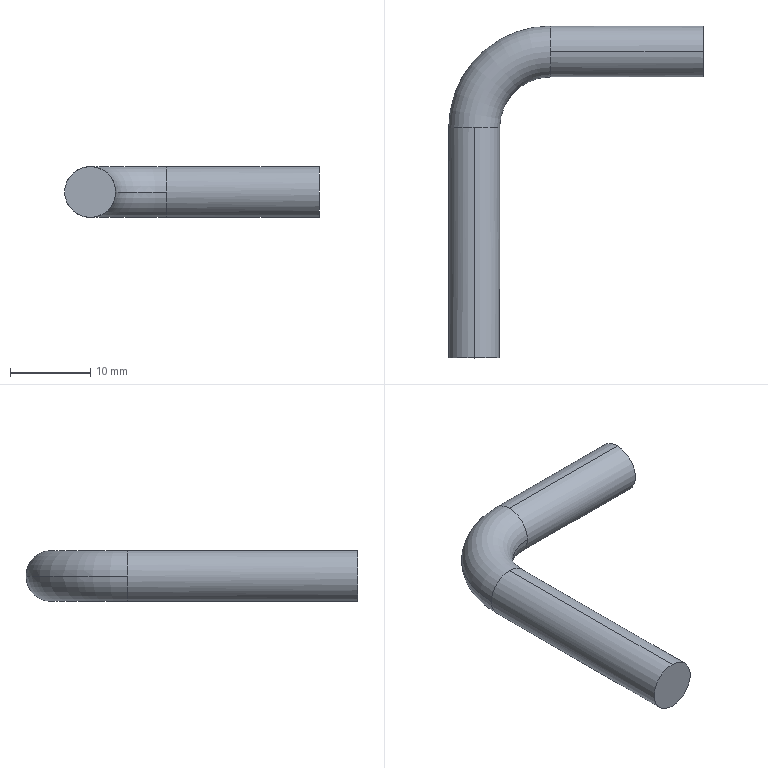Part | SolidWorks | features Sweep 1 | 1 solid | 8 faces | box 31.75 x 41.402 x 6.35 mm | volume 1986 mm3 | cylinder 4 | torus 2 | plane 2 | commonest cylinder face diameters 6.35 x4
STEP:
#1=CARTESIAN_POINT('',(0.,1.13,-0.125));
#2=VERTEX_POINT('',#1);
#3=CARTESIAN_POINT('',(-0.125,1.13,0.));
#4=VERTEX_POINT('',#3);
#5=CARTESIAN_POINT('',(0.,1.13,0.));
#6=DIRECTION('',(0.,1.,0.));
#7=DIRECTION('',(0.,0.,1.));
#8=AXIS2_PLACEMENT_3D('',#5,#6,#7);
#9=CIRCLE('',#8,0.125);
#10=EDGE_CURVE('',#2,#4,#9,.T.);
#11=ORIENTED_EDGE('',*,*,#10,.T.);
#12=CARTESIAN_POINT('',(0.375,1.63,0.));
#13=VERTEX_POINT('',#12);
#14=CARTESIAN_POINT('',(0.375,1.13,0.));
#15=DIRECTION('',(0.,0.,-1.));
#16=DIRECTION('',(-1.,0.,0.));
#17=AXIS2_PLACEMENT_3D('',#14,#15,#16);
#18=CIRCLE('',#17,0.5);
#19=EDGE_CURVE('',#4,#13,#18,.T.);
#20=ORIENTED_EDGE('',*,*,#19,.T.);
#21=CARTESIAN_POINT('',(0.375,1.505,-0.125));
#22=VERTEX_POINT('',#21);
#23=CARTESIAN_POINT('',(0.375,1.505,0.));
#24=DIRECTION('',(1.,0.,0.));
#25=DIRECTION('',(0.,0.,1.));
#26=AXIS2_PLACEMENT_3D('',#23,#24,#25);
#27=CIRCLE('',#26,0.125);
#28=EDGE_CURVE('',#22,#13,#27,.T.);
#29=ORIENTED_EDGE('',*,*,#28,.F.);
#30=CARTESIAN_POINT('',(0.375,1.38,0.));
#31=VERTEX_POINT('',#30);
#32=CARTESIAN_POINT('',(0.375,1.505,0.));
#33=DIRECTION('',(1.,0.,0.));
#34=DIRECTION('',(0.,0.,1.));
#35=AXIS2_PLACEMENT_3D('',#32,#33,#34);
#36=CIRCLE('',#35,0.125);
#37=EDGE_CURVE('',#31,#22,#36,.T.);
#38=ORIENTED_EDGE('',*,*,#37,.F.);
#39=CARTESIAN_POINT('',(0.125,1.13,0.));
#40=VERTEX_POINT('',#39);
#41=CARTESIAN_POINT('',(0.375,1.13,0.));
#42=DIRECTION('',(0.,0.,-1.));
#43=DIRECTION('',(-1.,0.,0.));
#44=AXIS2_PLACEMENT_3D('',#41,#42,#43);
#45=CIRCLE('',#44,0.25);
#46=EDGE_CURVE('',#40,#31,#45,.T.);
#47=ORIENTED_EDGE('',*,*,#46,.F.);
#48=CARTESIAN_POINT('',(0.,1.13,0.));
#49=DIRECTION('',(0.,1.,0.));
#50=DIRECTION('',(0.,0.,1.));
#51=AXIS2_PLACEMENT_3D('',#48,#49,#50);
#52=CIRCLE('',#51,0.125);
#53=EDGE_CURVE('',#40,#2,#52,.T.);
#54=ORIENTED_EDGE('',*,*,#53,.T.);
#55=EDGE_LOOP('',(#11,#20,#29,#38,#47,#54));
#56=FACE_OUTER_BOUND('',#55,.T.);
#57=CARTESIAN_POINT('',(0.375,1.13,0.));
#58=DIRECTION('',(0.,0.,-1.));
#59=DIRECTION('',(-1.,0.,0.));
#60=AXIS2_PLACEMENT_3D('',#57,#58,#59);
#61=TOROIDAL_SURFACE('',#60,0.375,0.125);
#62=ADVANCED_FACE('',(#56),#61,.T.);
#63=CARTESIAN_POINT('',(0.,1.13,0.125));
#64=VERTEX_POINT('',#63);
#65=CARTESIAN_POINT('',(0.,1.13,0.));
#66=DIRECTION('',(0.,1.,0.));
#67=DIRECTION('',(0.,0.,1.));
#68=AXIS2_PLACEMENT_3D('',#65,#66,#67);
#69=CIRCLE('',#68,0.125);
#70=EDGE_CURVE('',#64,#40,#69,.T.);
#71=ORIENTED_EDGE('',*,*,#70,.F.);
#72=CARTESIAN_POINT('',(0.,0.,0.125));
#73=VERTEX_POINT('',#72);
#74=CARTESIAN_POINT('',(0.,1.13,0.125));
#75=DIRECTION('',(0.,-1.,0.));
#76=VECTOR('',#75,39.37);
#77=LINE('',#74,#76);
#78=EDGE_CURVE('',#64,#73,#77,.T.);
#79=ORIENTED_EDGE('',*,*,#78,.T.);
#80=CARTESIAN_POINT('',(0.,0.,-0.125));
#81=VERTEX_POINT('',#80);
#82=CARTESIAN_POINT('',(0.,0.,0.));
#83=DIRECTION('',(0.,1.,0.));
#84=DIRECTION('',(0.,0.,1.));
#85=AXIS2_PLACEMENT_3D('',#82,#83,#84);
#86=CIRCLE('',#85,0.125);
#87=EDGE_CURVE('',#73,#81,#86,.T.);
#88=ORIENTED_EDGE('',*,*,#87,.T.);
#89=CARTESIAN_POINT('',(0.,1.13,-0.125));
#90=DIRECTION('',(0.,-1.,0.));
#91=VECTOR('',#90,39.37);
#92=LINE('',#89,#91);
#93=EDGE_CURVE('',#2,#81,#92,.T.);
#94=ORIENTED_EDGE('',*,*,#93,.F.);
#95=ORIENTED_EDGE('',*,*,#53,.F.);
#96=EDGE_LOOP('',(#71,#79,#88,#94,#95));
#97=FACE_OUTER_BOUND('',#96,.T.);
#98=CARTESIAN_POINT('',(0.,1.13,0.));
#99=DIRECTION('',(0.,-1.,0.));
#100=DIRECTION('',(0.,0.,-1.));
#101=AXIS2_PLACEMENT_3D('',#98,#99,#100);
#102=CYLINDRICAL_SURFACE('',#101,0.125);
#103=ADVANCED_FACE('',(#97),#102,.T.);
#104=ORIENTED_EDGE('',*,*,#28,.T.);
#105=CARTESIAN_POINT('',(0.375,1.505,0.125));
#106=VERTEX_POINT('',#105);
#107=CARTESIAN_POINT('',(0.375,1.505,0.));
#108=DIRECTION('',(1.,0.,0.));
#109=DIRECTION('',(0.,0.,1.));
#110=AXIS2_PLACEMENT_3D('',#107,#108,#109);
#111=CIRCLE('',#110,0.125);
#112=EDGE_CURVE('',#13,#106,#111,.T.);
#113=ORIENTED_EDGE('',*,*,#112,.T.);
#114=CARTESIAN_POINT('',(1.125,1.505,0.125));
#115=VERTEX_POINT('',#114);
#116=CARTESIAN_POINT('',(0.375,1.505,0.125));
#117=DIRECTION('',(1.,0.,0.));
#118=VECTOR('',#117,39.37);
#119=LINE('',#116,#118);
#120=EDGE_CURVE('',#106,#115,#119,.T.);
#121=ORIENTED_EDGE('',*,*,#120,.T.);
#122=CARTESIAN_POINT('',(1.125,1.505,-0.125));
#123=VERTEX_POINT('',#122);
#124=CARTESIAN_POINT('',(1.125,1.505,0.));
#125=DIRECTION('',(1.,0.,0.));
#126=DIRECTION('',(0.,0.,1.));
#127=AXIS2_PLACEMENT_3D('',#124,#125,#126);
#128=CIRCLE('',#127,0.125);
#129=EDGE_CURVE('',#123,#115,#128,.T.);
#130=ORIENTED_EDGE('',*,*,#129,.F.);
#131=CARTESIAN_POINT('',(0.375,1.505,-0.125));
#132=DIRECTION('',(1.,0.,0.));
#133=VECTOR('',#132,39.37);
#134=LINE('',#131,#133);
#135=EDGE_CURVE('',#22,#123,#134,.T.);
#136=ORIENTED_EDGE('',*,*,#135,.F.);
#137=EDGE_LOOP('',(#104,#113,#121,#130,#136));
#138=FACE_OUTER_BOUND('',#137,.T.);
#139=CARTESIAN_POINT('',(0.375,1.505,0.));
#140=DIRECTION('',(1.,0.,0.));
#141=DIRECTION('',(0.,0.,-1.));
#142=AXIS2_PLACEMENT_3D('',#139,#140,#141);
#143=CYLINDRICAL_SURFACE('',#142,0.125);
#144=ADVANCED_FACE('',(#138),#143,.T.);
#145=ORIENTED_EDGE('',*,*,#120,.F.);
#146=CARTESIAN_POINT('',(0.375,1.505,0.));
#147=DIRECTION('',(1.,0.,0.));
#148=DIRECTION('',(0.,0.,1.));
#149=AXIS2_PLACEMENT_3D('',#146,#147,#148);
#150=CIRCLE('',#149,0.125);
#151=EDGE_CURVE('',#106,#31,#150,.T.);
#152=ORIENTED_EDGE('',*,*,#151,.T.);
#153=ORIENTED_EDGE('',*,*,#37,.T.);
#154=ORIENTED_EDGE('',*,*,#135,.T.);
#155=CARTESIAN_POINT('',(1.125,1.505,0.));
#156=DIRECTION('',(1.,0.,0.));
#157=DIRECTION('',(0.,0.,1.));
#158=AXIS2_PLACEMENT_3D('',#155,#156,#157);
#159=CIRCLE('',#158,0.125);
#160=EDGE_CURVE('',#115,#123,#159,.T.);
#161=ORIENTED_EDGE('',*,*,#160,.F.);
#162=EDGE_LOOP('',(#145,#152,#153,#154,#161));
#163=FACE_OUTER_BOUND('',#162,.T.);
#164=CARTESIAN_POINT('',(0.375,1.505,0.));
#165=DIRECTION('',(1.,0.,0.));
#166=DIRECTION('',(0.,0.,-1.));
#167=AXIS2_PLACEMENT_3D('',#164,#165,#166);
#168=CYLINDRICAL_SURFACE('',#167,0.125);
#169=ADVANCED_FACE('',(#163),#168,.T.);
#170=ORIENTED_EDGE('',*,*,#19,.F.);
#171=CARTESIAN_POINT('',(0.,1.13,0.));
#172=DIRECTION('',(0.,1.,0.));
#173=DIRECTION('',(0.,0.,1.));
#174=AXIS2_PLACEMENT_3D('',#171,#172,#173);
#175=CIRCLE('',#174,0.125);
#176=EDGE_CURVE('',#4,#64,#175,.T.);
#177=ORIENTED_EDGE('',*,*,#176,.T.);
#178=ORIENTED_EDGE('',*,*,#70,.T.);
#179=ORIENTED_EDGE('',*,*,#46,.T.);
#180=ORIENTED_EDGE('',*,*,#151,.F.);
#181=ORIENTED_EDGE('',*,*,#112,.F.);
#182=EDGE_LOOP('',(#170,#177,#178,#179,#180,#181));
#183=FACE_OUTER_BOUND('',#182,.T.);
#184=CARTESIAN_POINT('',(0.375,1.13,0.));
#185=DIRECTION('',(0.,0.,-1.));
#186=DIRECTION('',(-1.,0.,0.));
#187=AXIS2_PLACEMENT_3D('',#184,#185,#186);
#188=TOROIDAL_SURFACE('',#187,0.375,0.125);
#189=ADVANCED_FACE('',(#183),#188,.T.);
#190=ORIENTED_EDGE('',*,*,#78,.F.);
#191=ORIENTED_EDGE('',*,*,#176,.F.);
#192=ORIENTED_EDGE('',*,*,#10,.F.);
#193=ORIENTED_EDGE('',*,*,#93,.T.);
#194=CARTESIAN_POINT('',(0.,0.,0.));
#195=DIRECTION('',(0.,1.,0.));
#196=DIRECTION('',(0.,0.,1.));
#197=AXIS2_PLACEMENT_3D('',#194,#195,#196);
#198=CIRCLE('',#197,0.125);
#199=EDGE_CURVE('',#81,#73,#198,.T.);
#200=ORIENTED_EDGE('',*,*,#199,.T.);
#201=EDGE_LOOP('',(#190,#191,#192,#193,#200));
#202=FACE_OUTER_BOUND('',#201,.T.);
#203=CARTESIAN_POINT('',(0.,1.13,0.));
#204=DIRECTION('',(0.,-1.,0.));
#205=DIRECTION('',(0.,0.,-1.));
#206=AXIS2_PLACEMENT_3D('',#203,#204,#205);
#207=CYLINDRICAL_SURFACE('',#206,0.125);
#208=ADVANCED_FACE('',(#202),#207,.T.);
#209=ORIENTED_EDGE('',*,*,#129,.T.);
#210=ORIENTED_EDGE('',*,*,#160,.T.);
#211=EDGE_LOOP('',(#209,#210));
#212=FACE_OUTER_BOUND('',#211,.T.);
#213=CARTESIAN_POINT('',(1.125,1.505,0.));
#214=DIRECTION('',(1.,0.,0.));
#215=DIRECTION('',(0.,0.,1.));
#216=AXIS2_PLACEMENT_3D('',#213,#214,#215);
#217=PLANE('',#216);
#218=ADVANCED_FACE('',(#212),#217,.T.);
#219=ORIENTED_EDGE('',*,*,#199,.F.);
#220=ORIENTED_EDGE('',*,*,#87,.F.);
#221=EDGE_LOOP('',(#219,#220));
#222=FACE_OUTER_BOUND('',#221,.T.);
#223=CARTESIAN_POINT('',(0.,0.,0.));
#224=DIRECTION('',(0.,1.,0.));
#225=DIRECTION('',(0.,0.,1.));
#226=AXIS2_PLACEMENT_3D('',#223,#224,#225);
#227=PLANE('',#226);
#228=ADVANCED_FACE('',(#222),#227,.F.);
#229=CLOSED_SHELL('',(#62,#103,#144,#169,#189,#208,#218,#228));
#230=MANIFOLD_SOLID_BREP('',#229);
#231=CARTESIAN_POINT('',(0.,0.,0.));
#232=DIRECTION('',(0.,0.,1.));
#233=DIRECTION('',(1.,0.,0.));
#234=AXIS2_PLACEMENT_3D('',#231,#232,#233);
#235=(LENGTH_UNIT()NAMED_UNIT(*)SI_UNIT($,.METRE.));
#236=LENGTH_MEASURE_WITH_UNIT(LENGTH_MEASURE(0.0254),#235);
#237=DIMENSIONAL_EXPONENTS(1.,0.,0.,0.,0.,0.,0.);
#238=(CONVERSION_BASED_UNIT('INCH',#236)LENGTH_UNIT()NAMED_UNIT(#237));
#239=UNCERTAINTY_MEASURE_WITH_UNIT(LENGTH_MEASURE(0.00001),#238,'','');
#240=(NAMED_UNIT(*)PLANE_ANGLE_UNIT()SI_UNIT($,.RADIAN.));
#241=(NAMED_UNIT(*)SI_UNIT($,.STERADIAN.)SOLID_ANGLE_UNIT());
#242=(GEOMETRIC_REPRESENTATION_CONTEXT(3)GLOBAL_UNCERTAINTY_ASSIGNED_CONTEXT((#239))GLOBAL_UNIT_ASSIGNED_CONTEXT((#238,#240,#241))REPRESENTATION_CONTEXT('',''));
#243=ADVANCED_BREP_SHAPE_REPRESENTATION('',(#230,#234),#242);